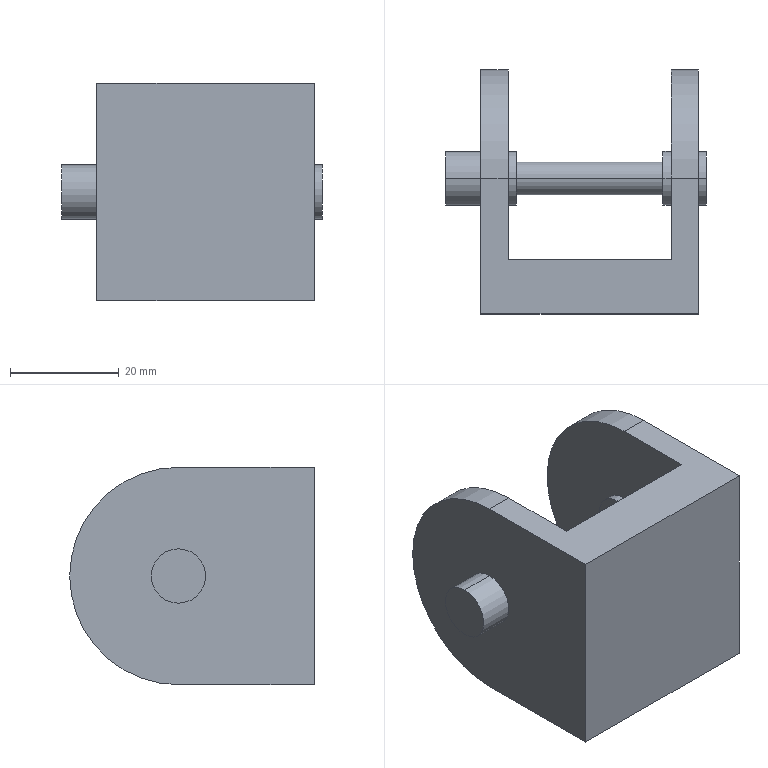Part | SolidWorks | features ICE 4, MirrorPattern 2, Extrusion 1 | 2 solids | 26 faces | box 48 x 45 x 40 mm | volume 29911 mm3 | plane 14 | cylinder 12 | commonest cylinder face diameters 10 x8 6 x2 40 x2
STEP:
#1=CARTESIAN_POINT('',(-13.5,25.,3.));
#2=VERTEX_POINT('',#1);
#3=CARTESIAN_POINT('',(-13.5,25.,-3.));
#4=VERTEX_POINT('',#3);
#5=CARTESIAN_POINT('',(-13.5,25.,0.));
#6=DIRECTION('',(-1.,0.,0.));
#7=DIRECTION('',(0.,0.,1.));
#8=AXIS2_PLACEMENT_3D('',#5,#6,#7);
#9=CIRCLE('',#8,3.);
#10=EDGE_CURVE('',#2,#4,#9,.T.);
#11=ORIENTED_EDGE('',*,*,#10,.F.);
#12=CARTESIAN_POINT('',(13.5,25.,3.));
#13=VERTEX_POINT('',#12);
#14=CARTESIAN_POINT('',(-21.502,25.,3.));
#15=DIRECTION('',(1.,0.,0.));
#16=VECTOR('',#15,1000.);
#17=LINE('',#14,#16);
#18=EDGE_CURVE('',#2,#13,#17,.T.);
#19=ORIENTED_EDGE('',*,*,#18,.T.);
#20=CARTESIAN_POINT('',(13.5,25.,-3.));
#21=VERTEX_POINT('',#20);
#22=CARTESIAN_POINT('',(13.5,25.,0.));
#23=DIRECTION('',(-1.,0.,0.));
#24=DIRECTION('',(0.,0.,1.));
#25=AXIS2_PLACEMENT_3D('',#22,#23,#24);
#26=CIRCLE('',#25,3.);
#27=EDGE_CURVE('',#13,#21,#26,.T.);
#28=ORIENTED_EDGE('',*,*,#27,.T.);
#29=CARTESIAN_POINT('',(-21.502,25.,-3.));
#30=DIRECTION('',(1.,0.,0.));
#31=VECTOR('',#30,1000.);
#32=LINE('',#29,#31);
#33=EDGE_CURVE('',#4,#21,#32,.T.);
#34=ORIENTED_EDGE('',*,*,#33,.F.);
#35=EDGE_LOOP('',(#11,#19,#28,#34));
#36=FACE_OUTER_BOUND('',#35,.T.);
#37=CARTESIAN_POINT('',(-21.502,25.,0.));
#38=DIRECTION('',(1.,0.,0.));
#39=DIRECTION('',(0.,0.,-1.));
#40=AXIS2_PLACEMENT_3D('',#37,#38,#39);
#41=CYLINDRICAL_SURFACE('',#40,3.);
#42=ADVANCED_FACE('',(#36),#41,.T.);
#43=CARTESIAN_POINT('',(-13.5,25.,0.));
#44=DIRECTION('',(-1.,0.,0.));
#45=DIRECTION('',(0.,0.,1.));
#46=AXIS2_PLACEMENT_3D('',#43,#44,#45);
#47=CIRCLE('',#46,3.);
#48=EDGE_CURVE('',#4,#2,#47,.T.);
#49=ORIENTED_EDGE('',*,*,#48,.T.);
#50=ORIENTED_EDGE('',*,*,#10,.T.);
#51=EDGE_LOOP('',(#49,#50));
#52=FACE_OUTER_BOUND('',#51,.T.);
#53=CARTESIAN_POINT('',(-13.5,25.,0.));
#54=DIRECTION('',(-1.,0.,0.));
#55=DIRECTION('',(0.,0.,-1.));
#56=AXIS2_PLACEMENT_3D('',#53,#54,#55);
#57=PLANE('',#56);
#58=ADVANCED_FACE('',(#52),#57,.T.);
#59=CARTESIAN_POINT('',(13.5,25.,0.));
#60=DIRECTION('',(-1.,0.,0.));
#61=DIRECTION('',(0.,0.,1.));
#62=AXIS2_PLACEMENT_3D('',#59,#60,#61);
#63=CIRCLE('',#62,3.);
#64=EDGE_CURVE('',#21,#13,#63,.T.);
#65=ORIENTED_EDGE('',*,*,#64,.F.);
#66=ORIENTED_EDGE('',*,*,#27,.F.);
#67=EDGE_LOOP('',(#65,#66));
#68=FACE_OUTER_BOUND('',#67,.T.);
#69=CARTESIAN_POINT('',(13.5,25.,0.));
#70=DIRECTION('',(-1.,0.,0.));
#71=DIRECTION('',(0.,0.,1.));
#72=AXIS2_PLACEMENT_3D('',#69,#70,#71);
#73=PLANE('',#72);
#74=ADVANCED_FACE('',(#68),#73,.F.);
#75=ORIENTED_EDGE('',*,*,#18,.F.);
#76=ORIENTED_EDGE('',*,*,#48,.F.);
#77=ORIENTED_EDGE('',*,*,#33,.T.);
#78=ORIENTED_EDGE('',*,*,#64,.T.);
#79=EDGE_LOOP('',(#75,#76,#77,#78));
#80=FACE_OUTER_BOUND('',#79,.T.);
#81=CARTESIAN_POINT('',(-21.502,25.,0.));
#82=DIRECTION('',(1.,0.,0.));
#83=DIRECTION('',(0.,0.,-1.));
#84=AXIS2_PLACEMENT_3D('',#81,#82,#83);
#85=CYLINDRICAL_SURFACE('',#84,3.);
#86=ADVANCED_FACE('',(#80),#85,.T.);
#87=CLOSED_SHELL('',(#42,#58,#74,#86));
#88=MANIFOLD_SOLID_BREP('',#87);
#89=CARTESIAN_POINT('',(-26.5,25.,5.));
#90=VERTEX_POINT('',#89);
#91=CARTESIAN_POINT('',(-26.5,25.,-5.));
#92=VERTEX_POINT('',#91);
#93=CARTESIAN_POINT('',(-26.5,25.,0.));
#94=DIRECTION('',(-1.,0.,0.));
#95=DIRECTION('',(0.,0.,1.));
#96=AXIS2_PLACEMENT_3D('',#93,#94,#95);
#97=CIRCLE('',#96,5.);
#98=EDGE_CURVE('',#90,#92,#97,.T.);
#99=ORIENTED_EDGE('',*,*,#98,.F.);
#100=CARTESIAN_POINT('',(-20.,25.,5.));
#101=VERTEX_POINT('',#100);
#102=CARTESIAN_POINT('',(-21.5,25.,5.));
#103=DIRECTION('',(1.,0.,0.));
#104=VECTOR('',#103,1000.);
#105=LINE('',#102,#104);
#106=EDGE_CURVE('',#90,#101,#105,.T.);
#107=ORIENTED_EDGE('',*,*,#106,.T.);
#108=CARTESIAN_POINT('',(-20.,25.,-5.));
#109=VERTEX_POINT('',#108);
#110=CARTESIAN_POINT('',(-20.,25.,0.));
#111=DIRECTION('',(1.,0.,0.));
#112=DIRECTION('',(0.,0.,-1.));
#113=AXIS2_PLACEMENT_3D('',#110,#111,#112);
#114=CIRCLE('',#113,5.);
#115=EDGE_CURVE('',#109,#101,#114,.T.);
#116=ORIENTED_EDGE('',*,*,#115,.F.);
#117=CARTESIAN_POINT('',(-21.5,25.,-5.));
#118=DIRECTION('',(1.,0.,0.));
#119=VECTOR('',#118,1000.);
#120=LINE('',#117,#119);
#121=EDGE_CURVE('',#92,#109,#120,.T.);
#122=ORIENTED_EDGE('',*,*,#121,.F.);
#123=EDGE_LOOP('',(#99,#107,#116,#122));
#124=FACE_OUTER_BOUND('',#123,.T.);
#125=CARTESIAN_POINT('',(-21.5,25.,0.));
#126=DIRECTION('',(1.,0.,0.));
#127=DIRECTION('',(0.,0.,-1.));
#128=AXIS2_PLACEMENT_3D('',#125,#126,#127);
#129=CYLINDRICAL_SURFACE('',#128,5.);
#130=ADVANCED_FACE('',(#124),#129,.T.);
#131=CARTESIAN_POINT('',(-15.,25.,-5.));
#132=VERTEX_POINT('',#131);
#133=CARTESIAN_POINT('',(-15.,25.,5.));
#134=VERTEX_POINT('',#133);
#135=CARTESIAN_POINT('',(-15.,25.,0.));
#136=DIRECTION('',(1.,0.,0.));
#137=DIRECTION('',(0.,0.,-1.));
#138=AXIS2_PLACEMENT_3D('',#135,#136,#137);
#139=CIRCLE('',#138,5.);
#140=EDGE_CURVE('',#132,#134,#139,.T.);
#141=ORIENTED_EDGE('',*,*,#140,.T.);
#142=CARTESIAN_POINT('',(-13.5,25.,5.));
#143=VERTEX_POINT('',#142);
#144=CARTESIAN_POINT('',(-21.5,25.,5.));
#145=DIRECTION('',(1.,0.,0.));
#146=VECTOR('',#145,1000.);
#147=LINE('',#144,#146);
#148=EDGE_CURVE('',#134,#143,#147,.T.);
#149=ORIENTED_EDGE('',*,*,#148,.T.);
#150=CARTESIAN_POINT('',(-13.5,25.,-5.));
#151=VERTEX_POINT('',#150);
#152=CARTESIAN_POINT('',(-13.5,25.,0.));
#153=DIRECTION('',(1.,0.,0.));
#154=DIRECTION('',(0.,0.,-1.));
#155=AXIS2_PLACEMENT_3D('',#152,#153,#154);
#156=CIRCLE('',#155,5.);
#157=EDGE_CURVE('',#151,#143,#156,.T.);
#158=ORIENTED_EDGE('',*,*,#157,.F.);
#159=CARTESIAN_POINT('',(-21.5,25.,-5.));
#160=DIRECTION('',(1.,0.,0.));
#161=VECTOR('',#160,1000.);
#162=LINE('',#159,#161);
#163=EDGE_CURVE('',#132,#151,#162,.T.);
#164=ORIENTED_EDGE('',*,*,#163,.F.);
#165=EDGE_LOOP('',(#141,#149,#158,#164));
#166=FACE_OUTER_BOUND('',#165,.T.);
#167=CARTESIAN_POINT('',(-21.5,25.,0.));
#168=DIRECTION('',(1.,0.,0.));
#169=DIRECTION('',(0.,0.,-1.));
#170=AXIS2_PLACEMENT_3D('',#167,#168,#169);
#171=CYLINDRICAL_SURFACE('',#170,5.);
#172=ADVANCED_FACE('',(#166),#171,.T.);
#173=CARTESIAN_POINT('',(21.5,25.,-5.));
#174=VERTEX_POINT('',#173);
#175=CARTESIAN_POINT('',(21.5,25.,5.));
#176=VERTEX_POINT('',#175);
#177=CARTESIAN_POINT('',(21.5,25.,0.));
#178=DIRECTION('',(1.,0.,0.));
#179=DIRECTION('',(0.,0.,-1.));
#180=AXIS2_PLACEMENT_3D('',#177,#178,#179);
#181=CIRCLE('',#180,5.);
#182=EDGE_CURVE('',#174,#176,#181,.T.);
#183=ORIENTED_EDGE('',*,*,#182,.F.);
#184=CARTESIAN_POINT('',(20.,25.,-5.));
#185=VERTEX_POINT('',#184);
#186=CARTESIAN_POINT('',(21.5,25.,-5.));
#187=DIRECTION('',(-1.,0.,0.));
#188=VECTOR('',#187,1000.);
#189=LINE('',#186,#188);
#190=EDGE_CURVE('',#174,#185,#189,.T.);
#191=ORIENTED_EDGE('',*,*,#190,.T.);
#192=CARTESIAN_POINT('',(20.,25.,5.));
#193=VERTEX_POINT('',#192);
#194=CARTESIAN_POINT('',(20.,25.,0.));
#195=DIRECTION('',(1.,0.,0.));
#196=DIRECTION('',(0.,0.,1.));
#197=AXIS2_PLACEMENT_3D('',#194,#195,#196);
#198=CIRCLE('',#197,5.);
#199=EDGE_CURVE('',#185,#193,#198,.T.);
#200=ORIENTED_EDGE('',*,*,#199,.T.);
#201=CARTESIAN_POINT('',(21.5,25.,5.));
#202=DIRECTION('',(-1.,0.,0.));
#203=VECTOR('',#202,1000.);
#204=LINE('',#201,#203);
#205=EDGE_CURVE('',#176,#193,#204,.T.);
#206=ORIENTED_EDGE('',*,*,#205,.F.);
#207=EDGE_LOOP('',(#183,#191,#200,#206));
#208=FACE_OUTER_BOUND('',#207,.T.);
#209=CARTESIAN_POINT('',(21.5,25.,0.));
#210=DIRECTION('',(-1.,0.,0.));
#211=DIRECTION('',(0.,0.,1.));
#212=AXIS2_PLACEMENT_3D('',#209,#210,#211);
#213=CYLINDRICAL_SURFACE('',#212,5.);
#214=ADVANCED_FACE('',(#208),#213,.T.);
#215=CARTESIAN_POINT('',(15.,25.,-5.));
#216=VERTEX_POINT('',#215);
#217=CARTESIAN_POINT('',(15.,25.,5.));
#218=VERTEX_POINT('',#217);
#219=CARTESIAN_POINT('',(15.,25.,0.));
#220=DIRECTION('',(1.,0.,0.));
#221=DIRECTION('',(0.,0.,1.));
#222=AXIS2_PLACEMENT_3D('',#219,#220,#221);
#223=CIRCLE('',#222,5.);
#224=EDGE_CURVE('',#216,#218,#223,.T.);
#225=ORIENTED_EDGE('',*,*,#224,.F.);
#226=CARTESIAN_POINT('',(13.5,25.,-5.));
#227=VERTEX_POINT('',#226);
#228=CARTESIAN_POINT('',(21.5,25.,-5.));
#229=DIRECTION('',(-1.,0.,0.));
#230=VECTOR('',#229,1000.);
#231=LINE('',#228,#230);
#232=EDGE_CURVE('',#216,#227,#231,.T.);
#233=ORIENTED_EDGE('',*,*,#232,.T.);
#234=CARTESIAN_POINT('',(13.5,25.,5.));
#235=VERTEX_POINT('',#234);
#236=CARTESIAN_POINT('',(13.5,25.,0.));
#237=DIRECTION('',(1.,0.,0.));
#238=DIRECTION('',(0.,0.,-1.));
#239=AXIS2_PLACEMENT_3D('',#236,#237,#238);
#240=CIRCLE('',#239,5.);
#241=EDGE_CURVE('',#227,#235,#240,.T.);
#242=ORIENTED_EDGE('',*,*,#241,.T.);
#243=CARTESIAN_POINT('',(21.5,25.,5.));
#244=DIRECTION('',(-1.,0.,0.));
#245=VECTOR('',#244,1000.);
#246=LINE('',#243,#245);
#247=EDGE_CURVE('',#218,#235,#246,.T.);
#248=ORIENTED_EDGE('',*,*,#247,.F.);
#249=EDGE_LOOP('',(#225,#233,#242,#248));
#250=FACE_OUTER_BOUND('',#249,.T.);
#251=CARTESIAN_POINT('',(21.5,25.,0.));
#252=DIRECTION('',(-1.,0.,0.));
#253=DIRECTION('',(0.,0.,1.));
#254=AXIS2_PLACEMENT_3D('',#251,#252,#253);
#255=CYLINDRICAL_SURFACE('',#254,5.);
#256=ADVANCED_FACE('',(#250),#255,.T.);
#257=CARTESIAN_POINT('',(-15.,10.,20.));
#258=VERTEX_POINT('',#257);
#259=CARTESIAN_POINT('',(-15.,10.,-20.));
#260=VERTEX_POINT('',#259);
#261=CARTESIAN_POINT('',(-15.,10.,20.));
#262=DIRECTION('',(0.,0.,-1.));
#263=VECTOR('',#262,1000.);
#264=LINE('',#261,#263);
#265=EDGE_CURVE('',#258,#260,#264,.T.);
#266=ORIENTED_EDGE('',*,*,#265,.F.);
#267=CARTESIAN_POINT('',(15.,10.,20.));
#268=VERTEX_POINT('',#267);
#269=CARTESIAN_POINT('',(-20.,10.,20.));
#270=DIRECTION('',(1.,0.,0.));
#271=VECTOR('',#270,1000.);
#272=LINE('',#269,#271);
#273=EDGE_CURVE('',#258,#268,#272,.T.);
#274=ORIENTED_EDGE('',*,*,#273,.T.);
#275=CARTESIAN_POINT('',(15.,10.,-20.));
#276=VERTEX_POINT('',#275);
#277=CARTESIAN_POINT('',(15.,10.,20.));
#278=DIRECTION('',(0.,0.,-1.));
#279=VECTOR('',#278,1000.);
#280=LINE('',#277,#279);
#281=EDGE_CURVE('',#268,#276,#280,.T.);
#282=ORIENTED_EDGE('',*,*,#281,.T.);
#283=CARTESIAN_POINT('',(-20.,10.,-20.));
#284=DIRECTION('',(-1.,0.,0.));
#285=VECTOR('',#284,1000.);
#286=LINE('',#283,#285);
#287=EDGE_CURVE('',#276,#260,#286,.T.);
#288=ORIENTED_EDGE('',*,*,#287,.T.);
#289=EDGE_LOOP('',(#266,#274,#282,#288));
#290=FACE_OUTER_BOUND('',#289,.T.);
#291=CARTESIAN_POINT('',(0.,10.,0.));
#292=DIRECTION('',(0.,1.,0.));
#293=DIRECTION('',(0.,0.,1.));
#294=AXIS2_PLACEMENT_3D('',#291,#292,#293);
#295=PLANE('',#294);
#296=ADVANCED_FACE('',(#290),#295,.T.);
#297=CARTESIAN_POINT('',(20.,25.,0.));
#298=DIRECTION('',(1.,0.,0.));
#299=DIRECTION('',(0.,0.,1.));
#300=AXIS2_PLACEMENT_3D('',#297,#298,#299);
#301=CIRCLE('',#300,5.);
#302=EDGE_CURVE('',#193,#185,#301,.T.);
#303=ORIENTED_EDGE('',*,*,#302,.F.);
#304=ORIENTED_EDGE('',*,*,#199,.F.);
#305=EDGE_LOOP('',(#303,#304));
#306=FACE_BOUND('',#305,.T.);
#307=CARTESIAN_POINT('',(20.,0.,20.));
#308=VERTEX_POINT('',#307);
#309=CARTESIAN_POINT('',(20.,0.,-20.));
#310=VERTEX_POINT('',#309);
#311=CARTESIAN_POINT('',(20.,0.,-20.));
#312=DIRECTION('',(0.,0.,-1.));
#313=VECTOR('',#312,1000.);
#314=LINE('',#311,#313);
#315=EDGE_CURVE('',#308,#310,#314,.T.);
#316=ORIENTED_EDGE('',*,*,#315,.T.);
#317=CARTESIAN_POINT('',(20.,25.,-20.));
#318=VERTEX_POINT('',#317);
#319=CARTESIAN_POINT('',(20.,10.,-20.));
#320=DIRECTION('',(0.,-1.,0.));
#321=VECTOR('',#320,1000.);
#322=LINE('',#319,#321);
#323=EDGE_CURVE('',#318,#310,#322,.T.);
#324=ORIENTED_EDGE('',*,*,#323,.F.);
#325=CARTESIAN_POINT('',(20.,25.,20.));
#326=VERTEX_POINT('',#325);
#327=CARTESIAN_POINT('',(20.,25.,0.));
#328=DIRECTION('',(1.,0.,0.));
#329=DIRECTION('',(0.,0.,1.));
#330=AXIS2_PLACEMENT_3D('',#327,#328,#329);
#331=CIRCLE('',#330,20.);
#332=EDGE_CURVE('',#318,#326,#331,.T.);
#333=ORIENTED_EDGE('',*,*,#332,.T.);
#334=CARTESIAN_POINT('',(20.,10.,20.));
#335=DIRECTION('',(0.,-1.,0.));
#336=VECTOR('',#335,1000.);
#337=LINE('',#334,#336);
#338=EDGE_CURVE('',#326,#308,#337,.T.);
#339=ORIENTED_EDGE('',*,*,#338,.T.);
#340=EDGE_LOOP('',(#316,#324,#333,#339));
#341=FACE_OUTER_BOUND('',#340,.T.);
#342=CARTESIAN_POINT('',(20.,10.,-20.));
#343=DIRECTION('',(-1.,0.,0.));
#344=DIRECTION('',(0.,0.,1.));
#345=AXIS2_PLACEMENT_3D('',#342,#343,#344);
#346=PLANE('',#345);
#347=ADVANCED_FACE('',(#306,#341),#346,.F.);
#348=CARTESIAN_POINT('',(-20.,0.,-20.));
#349=VERTEX_POINT('',#348);
#350=CARTESIAN_POINT('',(-20.,0.,-20.));
#351=DIRECTION('',(-1.,0.,0.));
#352=VECTOR('',#351,1000.);
#353=LINE('',#350,#352);
#354=EDGE_CURVE('',#310,#349,#353,.T.);
#355=ORIENTED_EDGE('',*,*,#354,.T.);
#356=CARTESIAN_POINT('',(-20.,25.,-20.));
#357=VERTEX_POINT('',#356);
#358=CARTESIAN_POINT('',(-20.,10.,-20.));
#359=DIRECTION('',(0.,-1.,0.));
#360=VECTOR('',#359,1000.);
#361=LINE('',#358,#360);
#362=EDGE_CURVE('',#357,#349,#361,.T.);
#363=ORIENTED_EDGE('',*,*,#362,.F.);
#364=CARTESIAN_POINT('',(-15.,25.,-20.));
#365=VERTEX_POINT('',#364);
#366=CARTESIAN_POINT('',(-15.,25.,-20.));
#367=DIRECTION('',(-1.,0.,0.));
#368=VECTOR('',#367,1000.);
#369=LINE('',#366,#368);
#370=EDGE_CURVE('',#365,#357,#369,.T.);
#371=ORIENTED_EDGE('',*,*,#370,.F.);
#372=CARTESIAN_POINT('',(-15.,10.,-20.));
#373=DIRECTION('',(0.,1.,0.));
#374=VECTOR('',#373,1000.);
#375=LINE('',#372,#374);
#376=EDGE_CURVE('',#260,#365,#375,.T.);
#377=ORIENTED_EDGE('',*,*,#376,.F.);
#378=ORIENTED_EDGE('',*,*,#287,.F.);
#379=CARTESIAN_POINT('',(15.,25.,-20.));
#380=VERTEX_POINT('',#379);
#381=CARTESIAN_POINT('',(15.,10.,-20.));
#382=DIRECTION('',(0.,1.,0.));
#383=VECTOR('',#382,1000.);
#384=LINE('',#381,#383);
#385=EDGE_CURVE('',#276,#380,#384,.T.);
#386=ORIENTED_EDGE('',*,*,#385,.T.);
#387=CARTESIAN_POINT('',(15.,25.,-20.));
#388=DIRECTION('',(1.,0.,0.));
#389=VECTOR('',#388,1000.);
#390=LINE('',#387,#389);
#391=EDGE_CURVE('',#380,#318,#390,.T.);
#392=ORIENTED_EDGE('',*,*,#391,.T.);
#393=ORIENTED_EDGE('',*,*,#323,.T.);
#394=EDGE_LOOP('',(#355,#363,#371,#377,#378,#386,#392,#393));
#395=FACE_OUTER_BOUND('',#394,.T.);
#396=CARTESIAN_POINT('',(-20.,10.,-20.));
#397=DIRECTION('',(0.,0.,1.));
#398=DIRECTION('',(1.,0.,0.));
#399=AXIS2_PLACEMENT_3D('',#396,#397,#398);
#400=PLANE('',#399);
#401=ADVANCED_FACE('',(#395),#400,.F.);
#402=ORIENTED_EDGE('',*,*,#115,.T.);
#403=CARTESIAN_POINT('',(-20.,25.,0.));
#404=DIRECTION('',(1.,0.,0.));
#405=DIRECTION('',(0.,0.,-1.));
#406=AXIS2_PLACEMENT_3D('',#403,#404,#405);
#407=CIRCLE('',#406,5.);
#408=EDGE_CURVE('',#101,#109,#407,.T.);
#409=ORIENTED_EDGE('',*,*,#408,.T.);
#410=EDGE_LOOP('',(#402,#409));
#411=FACE_BOUND('',#410,.T.);
#412=CARTESIAN_POINT('',(-20.,0.,20.));
#413=VERTEX_POINT('',#412);
#414=CARTESIAN_POINT('',(-20.,0.,-20.));
#415=DIRECTION('',(0.,0.,1.));
#416=VECTOR('',#415,1000.);
#417=LINE('',#414,#416);
#418=EDGE_CURVE('',#349,#413,#417,.T.);
#419=ORIENTED_EDGE('',*,*,#418,.T.);
#420=CARTESIAN_POINT('',(-20.,25.,20.));
#421=VERTEX_POINT('',#420);
#422=CARTESIAN_POINT('',(-20.,10.,20.));
#423=DIRECTION('',(0.,-1.,0.));
#424=VECTOR('',#423,1000.);
#425=LINE('',#422,#424);
#426=EDGE_CURVE('',#421,#413,#425,.T.);
#427=ORIENTED_EDGE('',*,*,#426,.F.);
#428=CARTESIAN_POINT('',(-20.,25.,0.));
#429=DIRECTION('',(1.,0.,0.));
#430=DIRECTION('',(0.,0.,1.));
#431=AXIS2_PLACEMENT_3D('',#428,#429,#430);
#432=CIRCLE('',#431,20.);
#433=EDGE_CURVE('',#357,#421,#432,.T.);
#434=ORIENTED_EDGE('',*,*,#433,.F.);
#435=ORIENTED_EDGE('',*,*,#362,.T.);
#436=EDGE_LOOP('',(#419,#427,#434,#435));
#437=FACE_OUTER_BOUND('',#436,.T.);
#438=CARTESIAN_POINT('',(-20.,10.,-20.));
#439=DIRECTION('',(1.,0.,0.));
#440=DIRECTION('',(0.,0.,-1.));
#441=AXIS2_PLACEMENT_3D('',#438,#439,#440);
#442=PLANE('',#441);
#443=ADVANCED_FACE('',(#411,#437),#442,.F.);
#444=CARTESIAN_POINT('',(-20.,0.,20.));
#445=DIRECTION('',(1.,0.,0.));
#446=VECTOR('',#445,1000.);
#447=LINE('',#444,#446);
#448=EDGE_CURVE('',#413,#308,#447,.T.);
#449=ORIENTED_EDGE('',*,*,#448,.T.);
#450=ORIENTED_EDGE('',*,*,#338,.F.);
#451=CARTESIAN_POINT('',(15.,25.,20.));
#452=VERTEX_POINT('',#451);
#453=CARTESIAN_POINT('',(15.,25.,20.));
#454=DIRECTION('',(1.,0.,0.));
#455=VECTOR('',#454,1000.);
#456=LINE('',#453,#455);
#457=EDGE_CURVE('',#452,#326,#456,.T.);
#458=ORIENTED_EDGE('',*,*,#457,.F.);
#459=CARTESIAN_POINT('',(15.,10.,20.));
#460=DIRECTION('',(0.,-1.,0.));
#461=VECTOR('',#460,1000.);
#462=LINE('',#459,#461);
#463=EDGE_CURVE('',#452,#268,#462,.T.);
#464=ORIENTED_EDGE('',*,*,#463,.T.);
#465=ORIENTED_EDGE('',*,*,#273,.F.);
#466=CARTESIAN_POINT('',(-15.,25.,20.));
#467=VERTEX_POINT('',#466);
#468=CARTESIAN_POINT('',(-15.,10.,20.));
#469=DIRECTION('',(0.,-1.,0.));
#470=VECTOR('',#469,1000.);
#471=LINE('',#468,#470);
#472=EDGE_CURVE('',#467,#258,#471,.T.);
#473=ORIENTED_EDGE('',*,*,#472,.F.);
#474=CARTESIAN_POINT('',(-15.,25.,20.));
#475=DIRECTION('',(-1.,0.,0.));
#476=VECTOR('',#475,1000.);
#477=LINE('',#474,#476);
#478=EDGE_CURVE('',#467,#421,#477,.T.);
#479=ORIENTED_EDGE('',*,*,#478,.T.);
#480=ORIENTED_EDGE('',*,*,#426,.T.);
#481=EDGE_LOOP('',(#449,#450,#458,#464,#465,#473,#479,#480));
#482=FACE_OUTER_BOUND('',#481,.T.);
#483=CARTESIAN_POINT('',(-20.,10.,20.));
#484=DIRECTION('',(0.,0.,-1.));
#485=DIRECTION('',(-1.,0.,0.));
#486=AXIS2_PLACEMENT_3D('',#483,#484,#485);
#487=PLANE('',#486);
#488=ADVANCED_FACE('',(#482),#487,.F.);
#489=ORIENTED_EDGE('',*,*,#315,.F.);
#490=ORIENTED_EDGE('',*,*,#448,.F.);
#491=ORIENTED_EDGE('',*,*,#418,.F.);
#492=ORIENTED_EDGE('',*,*,#354,.F.);
#493=EDGE_LOOP('',(#489,#490,#491,#492));
#494=FACE_OUTER_BOUND('',#493,.T.);
#495=CARTESIAN_POINT('',(0.,0.,0.));
#496=DIRECTION('',(0.,1.,0.));
#497=DIRECTION('',(0.,0.,1.));
#498=AXIS2_PLACEMENT_3D('',#495,#496,#497);
#499=PLANE('',#498);
#500=ADVANCED_FACE('',(#494),#499,.F.);
#501=ORIENTED_EDGE('',*,*,#332,.F.);
#502=ORIENTED_EDGE('',*,*,#391,.F.);
#503=CARTESIAN_POINT('',(15.,25.,0.));
#504=DIRECTION('',(1.,0.,0.));
#505=DIRECTION('',(0.,0.,1.));
#506=AXIS2_PLACEMENT_3D('',#503,#504,#505);
#507=CIRCLE('',#506,20.);
#508=EDGE_CURVE('',#380,#452,#507,.T.);
#509=ORIENTED_EDGE('',*,*,#508,.T.);
#510=ORIENTED_EDGE('',*,*,#457,.T.);
#511=EDGE_LOOP('',(#501,#502,#509,#510));
#512=FACE_OUTER_BOUND('',#511,.T.);
#513=CARTESIAN_POINT('',(15.,25.,0.));
#514=DIRECTION('',(1.,0.,0.));
#515=DIRECTION('',(0.,0.,-1.));
#516=AXIS2_PLACEMENT_3D('',#513,#514,#515);
#517=CYLINDRICAL_SURFACE('',#516,20.);
#518=ADVANCED_FACE('',(#512),#517,.T.);
#519=CARTESIAN_POINT('',(15.,25.,0.));
#520=DIRECTION('',(1.,0.,0.));
#521=DIRECTION('',(0.,0.,1.));
#522=AXIS2_PLACEMENT_3D('',#519,#520,#521);
#523=CIRCLE('',#522,5.);
#524=EDGE_CURVE('',#218,#216,#523,.T.);
#525=ORIENTED_EDGE('',*,*,#524,.T.);
#526=ORIENTED_EDGE('',*,*,#224,.T.);
#527=EDGE_LOOP('',(#525,#526));
#528=FACE_BOUND('',#527,.T.);
#529=ORIENTED_EDGE('',*,*,#281,.F.);
#530=ORIENTED_EDGE('',*,*,#463,.F.);
#531=ORIENTED_EDGE('',*,*,#508,.F.);
#532=ORIENTED_EDGE('',*,*,#385,.F.);
#533=EDGE_LOOP('',(#529,#530,#531,#532));
#534=FACE_OUTER_BOUND('',#533,.T.);
#535=CARTESIAN_POINT('',(15.,25.,0.));
#536=DIRECTION('',(-1.,0.,0.));
#537=DIRECTION('',(0.,0.,1.));
#538=AXIS2_PLACEMENT_3D('',#535,#536,#537);
#539=PLANE('',#538);
#540=ADVANCED_FACE('',(#528,#534),#539,.T.);
#541=ORIENTED_EDGE('',*,*,#433,.T.);
#542=ORIENTED_EDGE('',*,*,#478,.F.);
#543=CARTESIAN_POINT('',(-15.,25.,0.));
#544=DIRECTION('',(1.,0.,0.));
#545=DIRECTION('',(0.,0.,1.));
#546=AXIS2_PLACEMENT_3D('',#543,#544,#545);
#547=CIRCLE('',#546,20.);
#548=EDGE_CURVE('',#365,#467,#547,.T.);
#549=ORIENTED_EDGE('',*,*,#548,.F.);
#550=ORIENTED_EDGE('',*,*,#370,.T.);
#551=EDGE_LOOP('',(#541,#542,#549,#550));
#552=FACE_OUTER_BOUND('',#551,.T.);
#553=CARTESIAN_POINT('',(-15.,25.,0.));
#554=DIRECTION('',(-1.,0.,0.));
#555=DIRECTION('',(0.,0.,1.));
#556=AXIS2_PLACEMENT_3D('',#553,#554,#555);
#557=CYLINDRICAL_SURFACE('',#556,20.);
#558=ADVANCED_FACE('',(#552),#557,.T.);
#559=ORIENTED_EDGE('',*,*,#140,.F.);
#560=CARTESIAN_POINT('',(-15.,25.,0.));
#561=DIRECTION('',(1.,0.,0.));
#562=DIRECTION('',(0.,0.,-1.));
#563=AXIS2_PLACEMENT_3D('',#560,#561,#562);
#564=CIRCLE('',#563,5.);
#565=EDGE_CURVE('',#134,#132,#564,.T.);
#566=ORIENTED_EDGE('',*,*,#565,.F.);
#567=EDGE_LOOP('',(#559,#566));
#568=FACE_BOUND('',#567,.T.);
#569=ORIENTED_EDGE('',*,*,#265,.T.);
#570=ORIENTED_EDGE('',*,*,#376,.T.);
#571=ORIENTED_EDGE('',*,*,#548,.T.);
#572=ORIENTED_EDGE('',*,*,#472,.T.);
#573=EDGE_LOOP('',(#569,#570,#571,#572));
#574=FACE_OUTER_BOUND('',#573,.T.);
#575=CARTESIAN_POINT('',(-15.,25.,0.));
#576=DIRECTION('',(1.,0.,0.));
#577=DIRECTION('',(0.,0.,1.));
#578=AXIS2_PLACEMENT_3D('',#575,#576,#577);
#579=PLANE('',#578);
#580=ADVANCED_FACE('',(#568,#574),#579,.T.);
#581=CARTESIAN_POINT('',(13.5,25.,0.));
#582=DIRECTION('',(1.,0.,0.));
#583=DIRECTION('',(0.,0.,-1.));
#584=AXIS2_PLACEMENT_3D('',#581,#582,#583);
#585=CIRCLE('',#584,5.);
#586=EDGE_CURVE('',#235,#227,#585,.T.);
#587=ORIENTED_EDGE('',*,*,#586,.F.);
#588=ORIENTED_EDGE('',*,*,#241,.F.);
#589=EDGE_LOOP('',(#587,#588));
#590=FACE_OUTER_BOUND('',#589,.T.);
#591=CARTESIAN_POINT('',(13.5,25.,0.));
#592=DIRECTION('',(1.,0.,0.));
#593=DIRECTION('',(0.,0.,-1.));
#594=AXIS2_PLACEMENT_3D('',#591,#592,#593);
#595=PLANE('',#594);
#596=ADVANCED_FACE('',(#590),#595,.F.);
#597=ORIENTED_EDGE('',*,*,#232,.F.);
#598=ORIENTED_EDGE('',*,*,#524,.F.);
#599=ORIENTED_EDGE('',*,*,#247,.T.);
#600=ORIENTED_EDGE('',*,*,#586,.T.);
#601=EDGE_LOOP('',(#597,#598,#599,#600));
#602=FACE_OUTER_BOUND('',#601,.T.);
#603=CARTESIAN_POINT('',(21.5,25.,0.));
#604=DIRECTION('',(-1.,0.,0.));
#605=DIRECTION('',(0.,0.,1.));
#606=AXIS2_PLACEMENT_3D('',#603,#604,#605);
#607=CYLINDRICAL_SURFACE('',#606,5.);
#608=ADVANCED_FACE('',(#602),#607,.T.);
#609=ORIENTED_EDGE('',*,*,#190,.F.);
#610=CARTESIAN_POINT('',(21.5,25.,0.));
#611=DIRECTION('',(1.,0.,0.));
#612=DIRECTION('',(0.,0.,-1.));
#613=AXIS2_PLACEMENT_3D('',#610,#611,#612);
#614=CIRCLE('',#613,5.);
#615=EDGE_CURVE('',#176,#174,#614,.T.);
#616=ORIENTED_EDGE('',*,*,#615,.F.);
#617=ORIENTED_EDGE('',*,*,#205,.T.);
#618=ORIENTED_EDGE('',*,*,#302,.T.);
#619=EDGE_LOOP('',(#609,#616,#617,#618));
#620=FACE_OUTER_BOUND('',#619,.T.);
#621=CARTESIAN_POINT('',(21.5,25.,0.));
#622=DIRECTION('',(-1.,0.,0.));
#623=DIRECTION('',(0.,0.,1.));
#624=AXIS2_PLACEMENT_3D('',#621,#622,#623);
#625=CYLINDRICAL_SURFACE('',#624,5.);
#626=ADVANCED_FACE('',(#620),#625,.T.);
#627=ORIENTED_EDGE('',*,*,#615,.T.);
#628=ORIENTED_EDGE('',*,*,#182,.T.);
#629=EDGE_LOOP('',(#627,#628));
#630=FACE_OUTER_BOUND('',#629,.T.);
#631=CARTESIAN_POINT('',(21.5,25.,0.));
#632=DIRECTION('',(1.,0.,0.));
#633=DIRECTION('',(0.,0.,-1.));
#634=AXIS2_PLACEMENT_3D('',#631,#632,#633);
#635=PLANE('',#634);
#636=ADVANCED_FACE('',(#630),#635,.T.);
#637=ORIENTED_EDGE('',*,*,#157,.T.);
#638=CARTESIAN_POINT('',(-13.5,25.,0.));
#639=DIRECTION('',(1.,0.,0.));
#640=DIRECTION('',(0.,0.,-1.));
#641=AXIS2_PLACEMENT_3D('',#638,#639,#640);
#642=CIRCLE('',#641,5.);
#643=EDGE_CURVE('',#143,#151,#642,.T.);
#644=ORIENTED_EDGE('',*,*,#643,.T.);
#645=EDGE_LOOP('',(#637,#644));
#646=FACE_OUTER_BOUND('',#645,.T.);
#647=CARTESIAN_POINT('',(-13.5,25.,0.));
#648=DIRECTION('',(-1.,0.,0.));
#649=DIRECTION('',(0.,0.,-1.));
#650=AXIS2_PLACEMENT_3D('',#647,#648,#649);
#651=PLANE('',#650);
#652=ADVANCED_FACE('',(#646),#651,.F.);
#653=ORIENTED_EDGE('',*,*,#148,.F.);
#654=ORIENTED_EDGE('',*,*,#565,.T.);
#655=ORIENTED_EDGE('',*,*,#163,.T.);
#656=ORIENTED_EDGE('',*,*,#643,.F.);
#657=EDGE_LOOP('',(#653,#654,#655,#656));
#658=FACE_OUTER_BOUND('',#657,.T.);
#659=CARTESIAN_POINT('',(-21.5,25.,0.));
#660=DIRECTION('',(1.,0.,0.));
#661=DIRECTION('',(0.,0.,-1.));
#662=AXIS2_PLACEMENT_3D('',#659,#660,#661);
#663=CYLINDRICAL_SURFACE('',#662,5.);
#664=ADVANCED_FACE('',(#658),#663,.T.);
#665=ORIENTED_EDGE('',*,*,#106,.F.);
#666=CARTESIAN_POINT('',(-26.5,25.,0.));
#667=DIRECTION('',(-1.,0.,0.));
#668=DIRECTION('',(0.,0.,1.));
#669=AXIS2_PLACEMENT_3D('',#666,#667,#668);
#670=CIRCLE('',#669,5.);
#671=EDGE_CURVE('',#92,#90,#670,.T.);
#672=ORIENTED_EDGE('',*,*,#671,.F.);
#673=ORIENTED_EDGE('',*,*,#121,.T.);
#674=ORIENTED_EDGE('',*,*,#408,.F.);
#675=EDGE_LOOP('',(#665,#672,#673,#674));
#676=FACE_OUTER_BOUND('',#675,.T.);
#677=CARTESIAN_POINT('',(-21.5,25.,0.));
#678=DIRECTION('',(1.,0.,0.));
#679=DIRECTION('',(0.,0.,-1.));
#680=AXIS2_PLACEMENT_3D('',#677,#678,#679);
#681=CYLINDRICAL_SURFACE('',#680,5.);
#682=ADVANCED_FACE('',(#676),#681,.T.);
#683=ORIENTED_EDGE('',*,*,#671,.T.);
#684=ORIENTED_EDGE('',*,*,#98,.T.);
#685=EDGE_LOOP('',(#683,#684));
#686=FACE_OUTER_BOUND('',#685,.T.);
#687=CARTESIAN_POINT('',(-26.5,25.,0.));
#688=DIRECTION('',(-1.,0.,0.));
#689=DIRECTION('',(0.,0.,1.));
#690=AXIS2_PLACEMENT_3D('',#687,#688,#689);
#691=PLANE('',#690);
#692=ADVANCED_FACE('',(#686),#691,.T.);
#693=CLOSED_SHELL('',(#130,#172,#214,#256,#296,#347,#401,#443,#488,#500,#518,#540,#558,#580,#596,#608,#626,#636,#652,#664,#682,#692));
#694=MANIFOLD_SOLID_BREP('',#693);
#695=CARTESIAN_POINT('',(0.,0.,0.));
#696=DIRECTION('',(0.,0.,1.));
#697=DIRECTION('',(1.,0.,0.));
#698=AXIS2_PLACEMENT_3D('',#695,#696,#697);
#699=(LENGTH_UNIT()NAMED_UNIT(*)SI_UNIT(.MILLI.,.METRE.));
#700=UNCERTAINTY_MEASURE_WITH_UNIT(LENGTH_MEASURE(0.00001),#699,'','');
#701=(NAMED_UNIT(*)PLANE_ANGLE_UNIT()SI_UNIT($,.RADIAN.));
#702=(NAMED_UNIT(*)SI_UNIT($,.STERADIAN.)SOLID_ANGLE_UNIT());
#703=(GEOMETRIC_REPRESENTATION_CONTEXT(3)GLOBAL_UNCERTAINTY_ASSIGNED_CONTEXT((#700))GLOBAL_UNIT_ASSIGNED_CONTEXT((#699,#701,#702))REPRESENTATION_CONTEXT('',''));
#704=ADVANCED_BREP_SHAPE_REPRESENTATION('',(#88,#694,#698),#703);